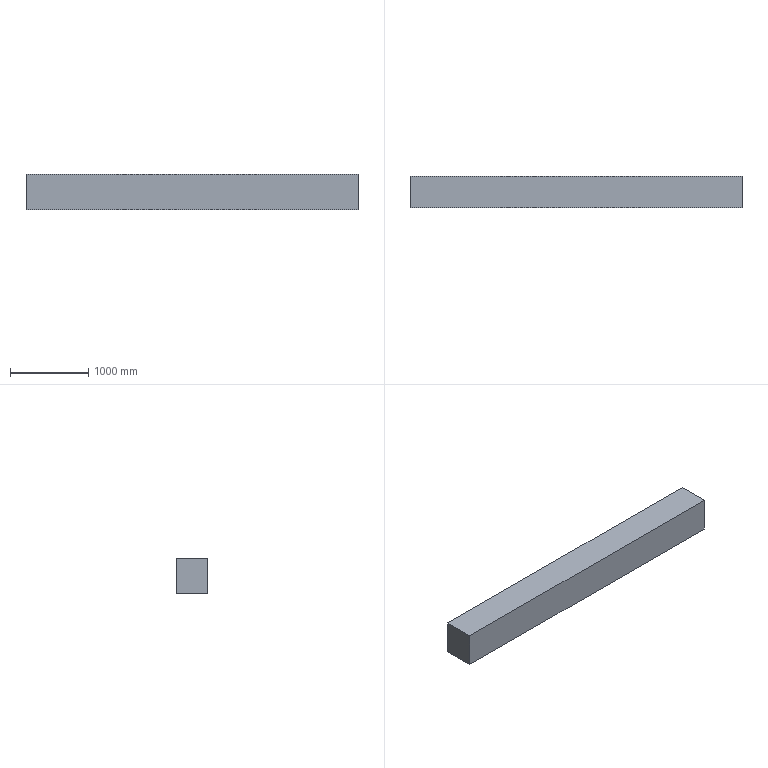Part | SolidWorks | features Extrusion 1 | 1 solid | 6 faces | box 4240 x 400 x 450 mm | volume 763200000 mm3 | plane 6
STEP:
#1=CARTESIAN_POINT('',(2120.,-200.,0.));
#2=VERTEX_POINT('',#1);
#3=CARTESIAN_POINT('',(2120.,200.,0.));
#4=VERTEX_POINT('',#3);
#5=CARTESIAN_POINT('',(2120.,200.,0.));
#6=DIRECTION('',(0.,1.,0.));
#7=VECTOR('',#6,1000.);
#8=LINE('',#5,#7);
#9=EDGE_CURVE('',#2,#4,#8,.T.);
#10=ORIENTED_EDGE('',*,*,#9,.T.);
#11=CARTESIAN_POINT('',(2120.,200.,450.));
#12=VERTEX_POINT('',#11);
#13=CARTESIAN_POINT('',(2120.,200.,450.));
#14=DIRECTION('',(0.,0.,-1.));
#15=VECTOR('',#14,1000.);
#16=LINE('',#13,#15);
#17=EDGE_CURVE('',#12,#4,#16,.T.);
#18=ORIENTED_EDGE('',*,*,#17,.F.);
#19=CARTESIAN_POINT('',(2120.,-200.,450.));
#20=VERTEX_POINT('',#19);
#21=CARTESIAN_POINT('',(2120.,200.,450.));
#22=DIRECTION('',(0.,1.,0.));
#23=VECTOR('',#22,1000.);
#24=LINE('',#21,#23);
#25=EDGE_CURVE('',#20,#12,#24,.T.);
#26=ORIENTED_EDGE('',*,*,#25,.F.);
#27=CARTESIAN_POINT('',(2120.,-200.,450.));
#28=DIRECTION('',(0.,0.,-1.));
#29=VECTOR('',#28,1000.);
#30=LINE('',#27,#29);
#31=EDGE_CURVE('',#20,#2,#30,.T.);
#32=ORIENTED_EDGE('',*,*,#31,.T.);
#33=EDGE_LOOP('',(#10,#18,#26,#32));
#34=FACE_OUTER_BOUND('',#33,.T.);
#35=CARTESIAN_POINT('',(2120.,200.,450.));
#36=DIRECTION('',(-1.,0.,0.));
#37=DIRECTION('',(0.,0.,1.));
#38=AXIS2_PLACEMENT_3D('',#35,#36,#37);
#39=PLANE('',#38);
#40=ADVANCED_FACE('',(#34),#39,.F.);
#41=CARTESIAN_POINT('',(-2120.,200.,0.));
#42=VERTEX_POINT('',#41);
#43=CARTESIAN_POINT('',(-2120.,200.,0.));
#44=DIRECTION('',(-1.,0.,0.));
#45=VECTOR('',#44,1000.);
#46=LINE('',#43,#45);
#47=EDGE_CURVE('',#4,#42,#46,.T.);
#48=ORIENTED_EDGE('',*,*,#47,.T.);
#49=CARTESIAN_POINT('',(-2120.,200.,450.));
#50=VERTEX_POINT('',#49);
#51=CARTESIAN_POINT('',(-2120.,200.,450.));
#52=DIRECTION('',(0.,0.,-1.));
#53=VECTOR('',#52,1000.);
#54=LINE('',#51,#53);
#55=EDGE_CURVE('',#50,#42,#54,.T.);
#56=ORIENTED_EDGE('',*,*,#55,.F.);
#57=CARTESIAN_POINT('',(-2120.,200.,450.));
#58=DIRECTION('',(-1.,0.,0.));
#59=VECTOR('',#58,1000.);
#60=LINE('',#57,#59);
#61=EDGE_CURVE('',#12,#50,#60,.T.);
#62=ORIENTED_EDGE('',*,*,#61,.F.);
#63=ORIENTED_EDGE('',*,*,#17,.T.);
#64=EDGE_LOOP('',(#48,#56,#62,#63));
#65=FACE_OUTER_BOUND('',#64,.T.);
#66=CARTESIAN_POINT('',(-2120.,200.,450.));
#67=DIRECTION('',(0.,-1.,0.));
#68=DIRECTION('',(0.,0.,-1.));
#69=AXIS2_PLACEMENT_3D('',#66,#67,#68);
#70=PLANE('',#69);
#71=ADVANCED_FACE('',(#65),#70,.F.);
#72=CARTESIAN_POINT('',(-2120.,-200.,0.));
#73=VERTEX_POINT('',#72);
#74=CARTESIAN_POINT('',(-2120.,200.,0.));
#75=DIRECTION('',(0.,-1.,0.));
#76=VECTOR('',#75,1000.);
#77=LINE('',#74,#76);
#78=EDGE_CURVE('',#42,#73,#77,.T.);
#79=ORIENTED_EDGE('',*,*,#78,.T.);
#80=CARTESIAN_POINT('',(-2120.,-200.,450.));
#81=VERTEX_POINT('',#80);
#82=CARTESIAN_POINT('',(-2120.,-200.,450.));
#83=DIRECTION('',(0.,0.,-1.));
#84=VECTOR('',#83,1000.);
#85=LINE('',#82,#84);
#86=EDGE_CURVE('',#81,#73,#85,.T.);
#87=ORIENTED_EDGE('',*,*,#86,.F.);
#88=CARTESIAN_POINT('',(-2120.,200.,450.));
#89=DIRECTION('',(0.,-1.,0.));
#90=VECTOR('',#89,1000.);
#91=LINE('',#88,#90);
#92=EDGE_CURVE('',#50,#81,#91,.T.);
#93=ORIENTED_EDGE('',*,*,#92,.F.);
#94=ORIENTED_EDGE('',*,*,#55,.T.);
#95=EDGE_LOOP('',(#79,#87,#93,#94));
#96=FACE_OUTER_BOUND('',#95,.T.);
#97=CARTESIAN_POINT('',(-2120.,200.,450.));
#98=DIRECTION('',(1.,0.,0.));
#99=DIRECTION('',(0.,0.,-1.));
#100=AXIS2_PLACEMENT_3D('',#97,#98,#99);
#101=PLANE('',#100);
#102=ADVANCED_FACE('',(#96),#101,.F.);
#103=CARTESIAN_POINT('',(-2120.,-200.,0.));
#104=DIRECTION('',(1.,0.,0.));
#105=VECTOR('',#104,1000.);
#106=LINE('',#103,#105);
#107=EDGE_CURVE('',#73,#2,#106,.T.);
#108=ORIENTED_EDGE('',*,*,#107,.T.);
#109=ORIENTED_EDGE('',*,*,#31,.F.);
#110=CARTESIAN_POINT('',(-2120.,-200.,450.));
#111=DIRECTION('',(1.,0.,0.));
#112=VECTOR('',#111,1000.);
#113=LINE('',#110,#112);
#114=EDGE_CURVE('',#81,#20,#113,.T.);
#115=ORIENTED_EDGE('',*,*,#114,.F.);
#116=ORIENTED_EDGE('',*,*,#86,.T.);
#117=EDGE_LOOP('',(#108,#109,#115,#116));
#118=FACE_OUTER_BOUND('',#117,.T.);
#119=CARTESIAN_POINT('',(-2120.,-200.,450.));
#120=DIRECTION('',(0.,1.,0.));
#121=DIRECTION('',(0.,0.,1.));
#122=AXIS2_PLACEMENT_3D('',#119,#120,#121);
#123=PLANE('',#122);
#124=ADVANCED_FACE('',(#118),#123,.F.);
#125=ORIENTED_EDGE('',*,*,#25,.T.);
#126=ORIENTED_EDGE('',*,*,#61,.T.);
#127=ORIENTED_EDGE('',*,*,#92,.T.);
#128=ORIENTED_EDGE('',*,*,#114,.T.);
#129=EDGE_LOOP('',(#125,#126,#127,#128));
#130=FACE_OUTER_BOUND('',#129,.T.);
#131=CARTESIAN_POINT('',(0.,0.,450.));
#132=DIRECTION('',(0.,0.,1.));
#133=DIRECTION('',(1.,0.,0.));
#134=AXIS2_PLACEMENT_3D('',#131,#132,#133);
#135=PLANE('',#134);
#136=ADVANCED_FACE('',(#130),#135,.T.);
#137=ORIENTED_EDGE('',*,*,#9,.F.);
#138=ORIENTED_EDGE('',*,*,#107,.F.);
#139=ORIENTED_EDGE('',*,*,#78,.F.);
#140=ORIENTED_EDGE('',*,*,#47,.F.);
#141=EDGE_LOOP('',(#137,#138,#139,#140));
#142=FACE_OUTER_BOUND('',#141,.T.);
#143=CARTESIAN_POINT('',(0.,0.,0.));
#144=DIRECTION('',(0.,0.,1.));
#145=DIRECTION('',(1.,0.,0.));
#146=AXIS2_PLACEMENT_3D('',#143,#144,#145);
#147=PLANE('',#146);
#148=ADVANCED_FACE('',(#142),#147,.F.);
#149=CLOSED_SHELL('',(#40,#71,#102,#124,#136,#148));
#150=MANIFOLD_SOLID_BREP('',#149);
#151=CARTESIAN_POINT('',(0.,0.,0.));
#152=DIRECTION('',(0.,0.,1.));
#153=DIRECTION('',(1.,0.,0.));
#154=AXIS2_PLACEMENT_3D('',#151,#152,#153);
#155=(LENGTH_UNIT()NAMED_UNIT(*)SI_UNIT(.MILLI.,.METRE.));
#156=UNCERTAINTY_MEASURE_WITH_UNIT(LENGTH_MEASURE(0.00001),#155,'','');
#157=(NAMED_UNIT(*)PLANE_ANGLE_UNIT()SI_UNIT($,.RADIAN.));
#158=(NAMED_UNIT(*)SI_UNIT($,.STERADIAN.)SOLID_ANGLE_UNIT());
#159=(GEOMETRIC_REPRESENTATION_CONTEXT(3)GLOBAL_UNCERTAINTY_ASSIGNED_CONTEXT((#156))GLOBAL_UNIT_ASSIGNED_CONTEXT((#155,#157,#158))REPRESENTATION_CONTEXT('',''));
#160=ADVANCED_BREP_SHAPE_REPRESENTATION('',(#150,#154),#159);